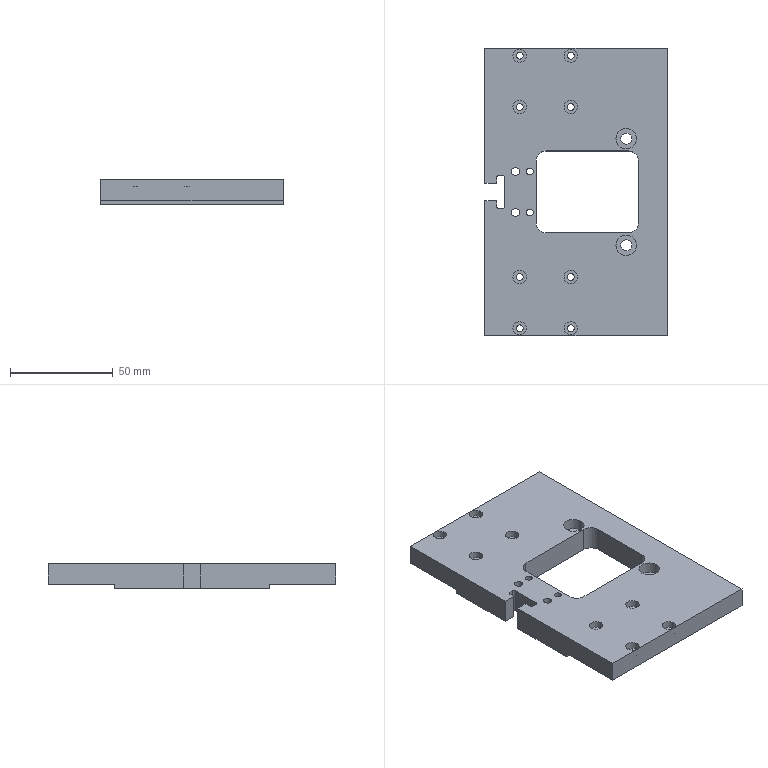Part | 1 solid | 68 faces | box 89 x 140 x 12 mm | volume 109630 mm3 | cylinder 34 | plane 32 | cone 2 | commonest cylinder face diameters 3.4 x8 6.5 x8 10 x6 2 x4 3.3 x2 4 x2